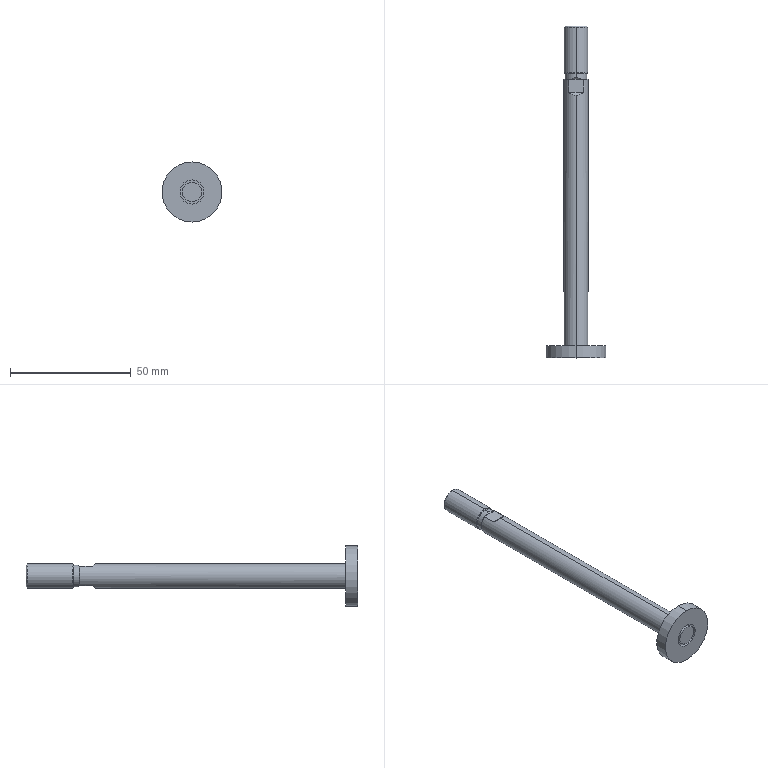Part | STEP file | 0229_Z_Cylinder_CG1BN25-50_3 | 1 solid | 32 faces | box 24.9 x 137.5 x 24.9 mm | volume 12725 mm3 | plane 14 | cylinder 12 | cone 6 | commonest cylinder face diameters 10 x6 8 x2 9.1 x2 24.9 x2